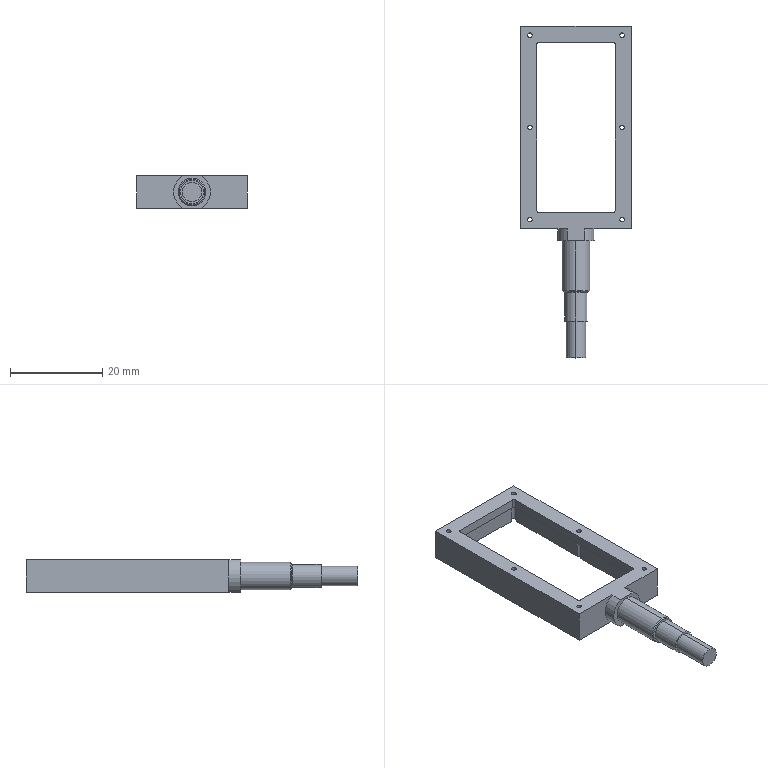CAM job | NX | 3-axis milling, drilling | part box 24 x 72 x 7 mm
Tools:
number,name,description,diameter,corner_radius,flute_length,length,flutes
11,D10JING,Milling Tool-5 Parameters,10.0,0.0,50.0,75.0,2
10,D10,Milling Tool-5 Parameters,10.0,0.0,50.0,75.0,2
7,D6A45,Milling Tool-5 Parameters,6.0,0.0,50.0,75.0,2
14,1.25ZT,Drilling Tool,1.25,0.0,35.0,50.0,2
13,1.0ZT,Drilling Tool,1.0,0.0,35.0,50.0,2
4,D4,Milling Tool-5 Parameters,4.0,0.0,50.0,75.0,2
2,D2,Milling Tool-5 Parameters,2.0,0.0,50.0,75.0,2
1,D1,Milling Tool-5 Parameters,1.0,0.0,50.0,75.0,2
Operations:
program,operation,operation_type,tool,method,geometry_group,spindle_rpm,surface_speed,feed_per_tooth,feed_cut,feed_plunge,cut_length_mm,path_length_mm,cut_time_min,machine_time_min
NONE,FLOOR_WALL_1,VolumeBased25DMillingOperation,D10JING,METHOD,A,9500.0,298.0,0.0658,1250.0,100.0,311.482,383.482,0.2492,0.2564
1,FLOOR_WALL,VolumeBased25DMillingOperation,D10,METHOD,A,9500.0,298.0,0.1316,2500.0,1000.0,4820.609,6184.946,2.083,2.22
1,DRILLING_COPY_1,Operation,D6A45,METHOD,A,5000.0,94.0,0.025,250.0,0.0,40.0,289.465,0.16,0.1849
1,DRILLING_COPY,Operation,1.25ZT,METHOD,A,2009.0,10.0,0.0249,100.0,0.0,30.502,218.584,0.305,0.3238
1,DRILLING_COPY_COPY,Operation,1.0ZT,METHOD,A,2009.0,10.0,0.0249,100.0,0.0,64.803,323.724,0.648,0.6739
1,CAVITY_MILL,CavityMilling,D10,METHOD,A,9500.0,298.0,0.1316,2500.0,1000.0,5346.996,5908.788,2.555,2.611
1,CAVITY_MILL_COPY,CavityMilling,D4,METHOD,A,9504.0,119.0,0.0868,1650.0,1000.0,770.056,1785.102,0.5362,0.6377
1,FLOOR_WALL_1_1,VolumeBased25DMillingOperation,D4,METHOD,A,9500.0,298.0,0.0658,1250.0,100.0,212.543,297.543,0.17,0.1785
1,ZLEVEL_PROFILE_COPY_1_COPY,ZLevelMilling,D4,METHOD,A,9500.0,298.0,0.0632,1200.0,1000.0,98.095,333.542,0.0826,0.1061
1,CAVITY_MILL_COPY_COPY,CavityMilling,D2,METHOD,A,9500.0,59.0,0.0579,1100.0,1000.0,1181.605,3529.273,1.108,1.343
1,CAVITY_MILL_COPY_COPY_COPY,CavityMilling,D1,METHOD,A,9500.0,29.0,0.0421,800.0,1000.0,1768.744,6471.391,2.066,2.537
1,PLANAR_MILL_COPY,PlanarMilling,D6A45,METHOD,A,9500.0,179.0,0.0658,1250.0,100.0,136.521,213.521,0.1092,0.1169
1,PLANAR_MILL_COPY_COPY,PlanarMilling,D6A45,METHOD,A,9500.0,179.0,0.0658,1250.0,100.0,120.583,197.583,0.0965,0.1042
1,刀补,VolumeBased25DMillingOperation,D4,METHOD,A,9500.0,298.0,0.0658,1250.0,100.0,111.061,196.061,0.0888,0.0973
2,FLOOR_WALL_COPY,VolumeBased25DMillingOperation,D10,METHOD,B,9500.0,298.0,0.1316,2500.0,1000.0,4820.609,5859.603,2.083,2.187
2,FLOOR_WALL_1_COPY,VolumeBased25DMillingOperation,D10JING,METHOD,B,9500.0,298.0,0.0658,1250.0,100.0,311.482,365.482,0.2492,0.2546
2,PLANAR_MILL_COPY_COPY_1,PlanarMilling,D6A45,METHOD,B,9500.0,179.0,0.0658,1250.0,100.0,132.521,191.521,0.106,0.1119
2,PLANAR_MILL_COPY_COPY_COPY,PlanarMilling,D6A45,METHOD,B,9500.0,179.0,0.0658,1250.0,100.0,108.311,167.311,0.0866,0.0925